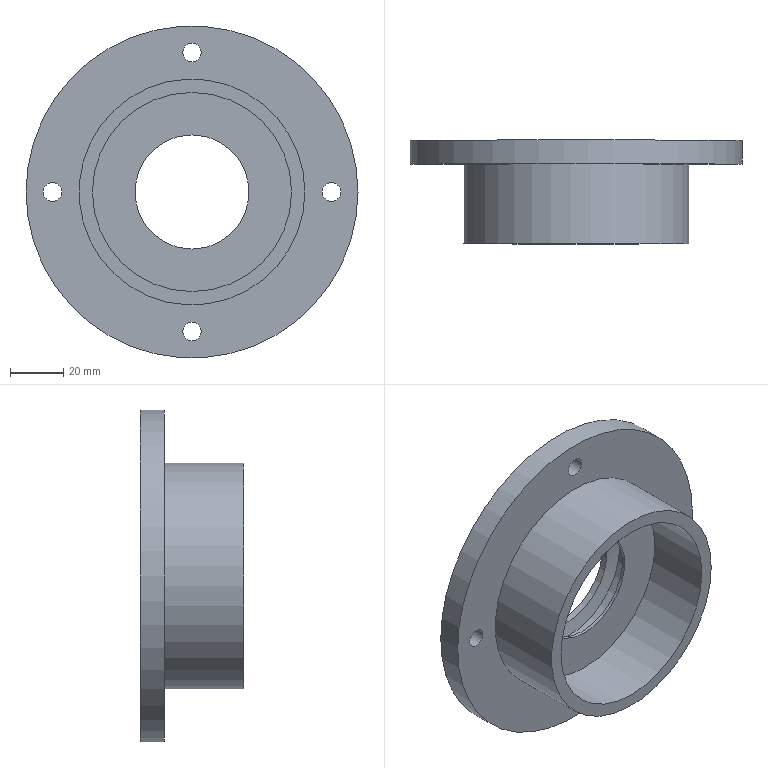Part | NX | features DATUM_CSYS 8, HOLE PACKAGE 7, SIMPLE HOLE 7, SKETCH 7, EXTRACT_DATUM_AXIS 4, Instance Feature 3, EXTRUDE 2, Pattern Feature 1, SWP104 1 | 1 solid | 18 faces | box 125 x 39 x 125 mm | volume 135227 mm3 | cylinder 11 | plane 5 | cone 2 | commonest cylinder face diameters 7 x4 43 x2 54 x1 75 x1 81 x1 85 x1
STEP:
#1=CARTESIAN_POINT('',(0.,-14.,21.5));
#2=VERTEX_POINT('',#1);
#3=CARTESIAN_POINT('',(0.,-14.,0.));
#4=DIRECTION('',(0.,1.,0.));
#5=DIRECTION('',(0.,0.,1.));
#6=AXIS2_PLACEMENT_3D('',#3,#4,#5);
#7=CIRCLE('',#6,21.5);
#8=EDGE_CURVE('',#2,#2,#7,.T.);
#9=ORIENTED_EDGE('',*,*,#8,.F.);
#10=EDGE_LOOP('',(#9));
#11=FACE_BOUND('',#10,.T.);
#12=CARTESIAN_POINT('',(0.,-12.735,21.5));
#13=VERTEX_POINT('',#12);
#14=CARTESIAN_POINT('',(0.,-12.735,0.));
#15=DIRECTION('',(0.,1.,0.));
#16=DIRECTION('',(0.,0.,1.));
#17=AXIS2_PLACEMENT_3D('',#14,#15,#16);
#18=CIRCLE('',#17,21.5);
#19=EDGE_CURVE('',#13,#13,#18,.F.);
#20=ORIENTED_EDGE('',*,*,#19,.F.);
#21=EDGE_LOOP('',(#20));
#22=FACE_BOUND('',#21,.T.);
#23=CARTESIAN_POINT('',(0.,0.,0.));
#24=DIRECTION('',(0.,-1.,0.));
#25=DIRECTION('',(0.,0.,-1.));
#26=AXIS2_PLACEMENT_3D('',#23,#24,#25);
#27=CYLINDRICAL_SURFACE('',#26,21.5);
#28=ADVANCED_FACE('',(#11,#22),#27,.F.);
#29=CARTESIAN_POINT('',(0.,-2.,-21.5));
#30=VERTEX_POINT('',#29);
#31=CARTESIAN_POINT('',(0.,-2.,0.));
#32=DIRECTION('',(0.,-1.,0.));
#33=DIRECTION('',(0.,0.,-1.));
#34=AXIS2_PLACEMENT_3D('',#31,#32,#33);
#35=CIRCLE('',#34,21.5);
#36=EDGE_CURVE('',#30,#30,#35,.T.);
#37=ORIENTED_EDGE('',*,*,#36,.F.);
#38=EDGE_LOOP('',(#37));
#39=FACE_BOUND('',#38,.T.);
#40=CARTESIAN_POINT('',(0.,-4.597,-21.5));
#41=VERTEX_POINT('',#40);
#42=CARTESIAN_POINT('',(0.,-4.597,0.));
#43=DIRECTION('',(0.,-1.,0.));
#44=DIRECTION('',(0.,0.,-1.));
#45=AXIS2_PLACEMENT_3D('',#42,#43,#44);
#46=CIRCLE('',#45,21.5);
#47=EDGE_CURVE('',#41,#41,#46,.F.);
#48=ORIENTED_EDGE('',*,*,#47,.F.);
#49=EDGE_LOOP('',(#48));
#50=FACE_BOUND('',#49,.T.);
#51=CARTESIAN_POINT('',(0.,0.,0.));
#52=DIRECTION('',(0.,-1.,0.));
#53=DIRECTION('',(0.,0.,-1.));
#54=AXIS2_PLACEMENT_3D('',#51,#52,#53);
#55=CYLINDRICAL_SURFACE('',#54,21.5);
#56=ADVANCED_FACE('',(#39,#50),#55,.F.);
#57=CARTESIAN_POINT('',(62.5,-9.,0.));
#58=VERTEX_POINT('',#57);
#59=CARTESIAN_POINT('',(0.,-9.,0.));
#60=DIRECTION('',(0.,-1.,0.));
#61=DIRECTION('',(1.,0.,0.));
#62=AXIS2_PLACEMENT_3D('',#59,#60,#61);
#63=CIRCLE('',#62,62.5);
#64=EDGE_CURVE('',#58,#58,#63,.T.);
#65=ORIENTED_EDGE('',*,*,#64,.F.);
#66=EDGE_LOOP('',(#65));
#67=FACE_BOUND('',#66,.T.);
#68=CARTESIAN_POINT('',(62.5,0.,0.));
#69=VERTEX_POINT('',#68);
#70=CARTESIAN_POINT('',(0.,0.,0.));
#71=DIRECTION('',(0.,-1.,0.));
#72=DIRECTION('',(1.,0.,0.));
#73=AXIS2_PLACEMENT_3D('',#70,#71,#72);
#74=CIRCLE('',#73,62.5);
#75=EDGE_CURVE('',#69,#69,#74,.T.);
#76=ORIENTED_EDGE('',*,*,#75,.T.);
#77=EDGE_LOOP('',(#76));
#78=FACE_BOUND('',#77,.T.);
#79=CARTESIAN_POINT('',(0.,-9.,0.));
#80=DIRECTION('',(0.,1.,0.));
#81=DIRECTION('',(0.,0.,1.));
#82=AXIS2_PLACEMENT_3D('',#79,#80,#81);
#83=CYLINDRICAL_SURFACE('',#82,62.5);
#84=ADVANCED_FACE('',(#67,#78),#83,.T.);
#85=CARTESIAN_POINT('',(0.,-9.,-56.));
#86=VERTEX_POINT('',#85);
#87=CARTESIAN_POINT('',(0.,-9.,-52.5));
#88=DIRECTION('',(0.,-1.,0.));
#89=DIRECTION('',(0.,0.,-1.));
#90=AXIS2_PLACEMENT_3D('',#87,#88,#89);
#91=CIRCLE('',#90,3.5);
#92=EDGE_CURVE('',#86,#86,#91,.T.);
#93=ORIENTED_EDGE('',*,*,#92,.F.);
#94=EDGE_LOOP('',(#93));
#95=FACE_BOUND('',#94,.T.);
#96=CARTESIAN_POINT('',(52.5,-9.,-3.5));
#97=VERTEX_POINT('',#96);
#98=CARTESIAN_POINT('',(52.5,-9.,0.));
#99=DIRECTION('',(0.,-1.,0.));
#100=DIRECTION('',(0.,0.,-1.));
#101=AXIS2_PLACEMENT_3D('',#98,#99,#100);
#102=CIRCLE('',#101,3.5);
#103=EDGE_CURVE('',#97,#97,#102,.T.);
#104=ORIENTED_EDGE('',*,*,#103,.F.);
#105=EDGE_LOOP('',(#104));
#106=FACE_BOUND('',#105,.T.);
#107=CARTESIAN_POINT('',(0.,-9.,49.));
#108=VERTEX_POINT('',#107);
#109=CARTESIAN_POINT('',(0.,-9.,52.5));
#110=DIRECTION('',(0.,-1.,0.));
#111=DIRECTION('',(0.,0.,-1.));
#112=AXIS2_PLACEMENT_3D('',#109,#110,#111);
#113=CIRCLE('',#112,3.5);
#114=EDGE_CURVE('',#108,#108,#113,.T.);
#115=ORIENTED_EDGE('',*,*,#114,.F.);
#116=EDGE_LOOP('',(#115));
#117=FACE_BOUND('',#116,.T.);
#118=CARTESIAN_POINT('',(-52.5,-9.,-3.5));
#119=VERTEX_POINT('',#118);
#120=CARTESIAN_POINT('',(-52.5,-9.,0.));
#121=DIRECTION('',(0.,-1.,0.));
#122=DIRECTION('',(0.,0.,-1.));
#123=AXIS2_PLACEMENT_3D('',#120,#121,#122);
#124=CIRCLE('',#123,3.5);
#125=EDGE_CURVE('',#119,#119,#124,.T.);
#126=ORIENTED_EDGE('',*,*,#125,.F.);
#127=EDGE_LOOP('',(#126));
#128=FACE_BOUND('',#127,.T.);
#129=CARTESIAN_POINT('',(42.5,-9.,0.));
#130=VERTEX_POINT('',#129);
#131=CARTESIAN_POINT('',(0.,-9.,0.));
#132=DIRECTION('',(0.,-1.,0.));
#133=DIRECTION('',(1.,0.,0.));
#134=AXIS2_PLACEMENT_3D('',#131,#132,#133);
#135=CIRCLE('',#134,42.5);
#136=EDGE_CURVE('',#130,#130,#135,.T.);
#137=ORIENTED_EDGE('',*,*,#136,.F.);
#138=EDGE_LOOP('',(#137));
#139=FACE_BOUND('',#138,.T.);
#140=ORIENTED_EDGE('',*,*,#64,.T.);
#141=EDGE_LOOP('',(#140));
#142=FACE_BOUND('',#141,.T.);
#143=CARTESIAN_POINT('',(0.,-9.,0.));
#144=DIRECTION('',(0.,-1.,0.));
#145=DIRECTION('',(0.,0.,-1.));
#146=AXIS2_PLACEMENT_3D('',#143,#144,#145);
#147=PLANE('',#146);
#148=ADVANCED_FACE('',(#95,#106,#117,#128,#139,#142),#147,.T.);
#149=CARTESIAN_POINT('',(0.,0.,-40.5));
#150=VERTEX_POINT('',#149);
#151=CARTESIAN_POINT('',(0.,0.,0.));
#152=DIRECTION('',(0.,-1.,0.));
#153=DIRECTION('',(0.,0.,-1.));
#154=AXIS2_PLACEMENT_3D('',#151,#152,#153);
#155=CIRCLE('',#154,40.5);
#156=EDGE_CURVE('',#150,#150,#155,.T.);
#157=ORIENTED_EDGE('',*,*,#156,.T.);
#158=EDGE_LOOP('',(#157));
#159=FACE_BOUND('',#158,.T.);
#160=CARTESIAN_POINT('',(0.,0.,-56.));
#161=VERTEX_POINT('',#160);
#162=CARTESIAN_POINT('',(0.,0.,-52.5));
#163=DIRECTION('',(0.,-1.,0.));
#164=DIRECTION('',(0.,0.,-1.));
#165=AXIS2_PLACEMENT_3D('',#162,#163,#164);
#166=CIRCLE('',#165,3.5);
#167=EDGE_CURVE('',#161,#161,#166,.T.);
#168=ORIENTED_EDGE('',*,*,#167,.T.);
#169=EDGE_LOOP('',(#168));
#170=FACE_BOUND('',#169,.T.);
#171=CARTESIAN_POINT('',(52.5,0.,-3.5));
#172=VERTEX_POINT('',#171);
#173=CARTESIAN_POINT('',(52.5,0.,0.));
#174=DIRECTION('',(0.,-1.,0.));
#175=DIRECTION('',(0.,0.,-1.));
#176=AXIS2_PLACEMENT_3D('',#173,#174,#175);
#177=CIRCLE('',#176,3.5);
#178=EDGE_CURVE('',#172,#172,#177,.T.);
#179=ORIENTED_EDGE('',*,*,#178,.T.);
#180=EDGE_LOOP('',(#179));
#181=FACE_BOUND('',#180,.T.);
#182=CARTESIAN_POINT('',(0.,0.,49.));
#183=VERTEX_POINT('',#182);
#184=CARTESIAN_POINT('',(0.,0.,52.5));
#185=DIRECTION('',(0.,-1.,0.));
#186=DIRECTION('',(0.,0.,-1.));
#187=AXIS2_PLACEMENT_3D('',#184,#185,#186);
#188=CIRCLE('',#187,3.5);
#189=EDGE_CURVE('',#183,#183,#188,.T.);
#190=ORIENTED_EDGE('',*,*,#189,.T.);
#191=EDGE_LOOP('',(#190));
#192=FACE_BOUND('',#191,.T.);
#193=CARTESIAN_POINT('',(-52.5,0.,-3.5));
#194=VERTEX_POINT('',#193);
#195=CARTESIAN_POINT('',(-52.5,0.,0.));
#196=DIRECTION('',(0.,-1.,0.));
#197=DIRECTION('',(0.,0.,-1.));
#198=AXIS2_PLACEMENT_3D('',#195,#196,#197);
#199=CIRCLE('',#198,3.5);
#200=EDGE_CURVE('',#194,#194,#199,.T.);
#201=ORIENTED_EDGE('',*,*,#200,.T.);
#202=EDGE_LOOP('',(#201));
#203=FACE_BOUND('',#202,.T.);
#204=ORIENTED_EDGE('',*,*,#75,.F.);
#205=EDGE_LOOP('',(#204));
#206=FACE_BOUND('',#205,.T.);
#207=CARTESIAN_POINT('',(0.,0.,0.));
#208=DIRECTION('',(0.,-1.,0.));
#209=DIRECTION('',(0.,0.,-1.));
#210=AXIS2_PLACEMENT_3D('',#207,#208,#209);
#211=PLANE('',#210);
#212=ADVANCED_FACE('',(#159,#170,#181,#192,#203,#206),#211,.F.);
#213=CARTESIAN_POINT('',(42.5,-39.,0.));
#214=VERTEX_POINT('',#213);
#215=CARTESIAN_POINT('',(0.,-39.,0.));
#216=DIRECTION('',(0.,-1.,0.));
#217=DIRECTION('',(1.,0.,0.));
#218=AXIS2_PLACEMENT_3D('',#215,#216,#217);
#219=CIRCLE('',#218,42.5);
#220=EDGE_CURVE('',#214,#214,#219,.T.);
#221=ORIENTED_EDGE('',*,*,#220,.F.);
#222=EDGE_LOOP('',(#221));
#223=FACE_BOUND('',#222,.T.);
#224=ORIENTED_EDGE('',*,*,#136,.T.);
#225=EDGE_LOOP('',(#224));
#226=FACE_BOUND('',#225,.T.);
#227=CARTESIAN_POINT('',(0.,-39.,0.));
#228=DIRECTION('',(0.,1.,0.));
#229=DIRECTION('',(0.,0.,1.));
#230=AXIS2_PLACEMENT_3D('',#227,#228,#229);
#231=CYLINDRICAL_SURFACE('',#230,42.5);
#232=ADVANCED_FACE('',(#223,#226),#231,.T.);
#233=CARTESIAN_POINT('',(0.,-39.,37.5));
#234=VERTEX_POINT('',#233);
#235=CARTESIAN_POINT('',(0.,-39.,0.));
#236=DIRECTION('',(0.,1.,0.));
#237=DIRECTION('',(0.,0.,1.));
#238=AXIS2_PLACEMENT_3D('',#235,#236,#237);
#239=CIRCLE('',#238,37.5);
#240=EDGE_CURVE('',#234,#234,#239,.T.);
#241=ORIENTED_EDGE('',*,*,#240,.T.);
#242=EDGE_LOOP('',(#241));
#243=FACE_BOUND('',#242,.T.);
#244=ORIENTED_EDGE('',*,*,#220,.T.);
#245=EDGE_LOOP('',(#244));
#246=FACE_BOUND('',#245,.T.);
#247=CARTESIAN_POINT('',(0.,-39.,0.));
#248=DIRECTION('',(0.,-1.,0.));
#249=DIRECTION('',(0.,0.,-1.));
#250=AXIS2_PLACEMENT_3D('',#247,#248,#249);
#251=PLANE('',#250);
#252=ADVANCED_FACE('',(#243,#246),#251,.T.);
#253=ORIENTED_EDGE('',*,*,#8,.T.);
#254=EDGE_LOOP('',(#253));
#255=FACE_BOUND('',#254,.T.);
#256=CARTESIAN_POINT('',(0.,-14.,37.5));
#257=VERTEX_POINT('',#256);
#258=CARTESIAN_POINT('',(0.,-14.,0.));
#259=DIRECTION('',(0.,1.,0.));
#260=DIRECTION('',(0.,0.,1.));
#261=AXIS2_PLACEMENT_3D('',#258,#259,#260);
#262=CIRCLE('',#261,37.5);
#263=EDGE_CURVE('',#257,#257,#262,.F.);
#264=ORIENTED_EDGE('',*,*,#263,.T.);
#265=EDGE_LOOP('',(#264));
#266=FACE_BOUND('',#265,.T.);
#267=CARTESIAN_POINT('',(0.,-14.,0.));
#268=DIRECTION('',(0.,1.,0.));
#269=DIRECTION('',(0.,0.,1.));
#270=AXIS2_PLACEMENT_3D('',#267,#268,#269);
#271=PLANE('',#270);
#272=ADVANCED_FACE('',(#255,#266),#271,.F.);
#273=ORIENTED_EDGE('',*,*,#263,.F.);
#274=EDGE_LOOP('',(#273));
#275=FACE_BOUND('',#274,.T.);
#276=ORIENTED_EDGE('',*,*,#240,.F.);
#277=EDGE_LOOP('',(#276));
#278=FACE_BOUND('',#277,.T.);
#279=CARTESIAN_POINT('',(0.,-39.,0.));
#280=DIRECTION('',(0.,1.,0.));
#281=DIRECTION('',(0.,0.,1.));
#282=AXIS2_PLACEMENT_3D('',#279,#280,#281);
#283=CYLINDRICAL_SURFACE('',#282,37.5);
#284=ADVANCED_FACE('',(#275,#278),#283,.F.);
#285=ORIENTED_EDGE('',*,*,#125,.T.);
#286=EDGE_LOOP('',(#285));
#287=FACE_BOUND('',#286,.T.);
#288=ORIENTED_EDGE('',*,*,#200,.F.);
#289=EDGE_LOOP('',(#288));
#290=FACE_BOUND('',#289,.T.);
#291=CARTESIAN_POINT('',(-52.5,0.,0.));
#292=DIRECTION('',(0.,-1.,0.));
#293=DIRECTION('',(0.,0.,-1.));
#294=AXIS2_PLACEMENT_3D('',#291,#292,#293);
#295=CYLINDRICAL_SURFACE('',#294,3.5);
#296=ADVANCED_FACE('',(#287,#290),#295,.F.);
#297=ORIENTED_EDGE('',*,*,#114,.T.);
#298=EDGE_LOOP('',(#297));
#299=FACE_BOUND('',#298,.T.);
#300=ORIENTED_EDGE('',*,*,#189,.F.);
#301=EDGE_LOOP('',(#300));
#302=FACE_BOUND('',#301,.T.);
#303=CARTESIAN_POINT('',(0.,0.,52.5));
#304=DIRECTION('',(0.,-1.,0.));
#305=DIRECTION('',(0.,0.,-1.));
#306=AXIS2_PLACEMENT_3D('',#303,#304,#305);
#307=CYLINDRICAL_SURFACE('',#306,3.5);
#308=ADVANCED_FACE('',(#299,#302),#307,.F.);
#309=ORIENTED_EDGE('',*,*,#103,.T.);
#310=EDGE_LOOP('',(#309));
#311=FACE_BOUND('',#310,.T.);
#312=ORIENTED_EDGE('',*,*,#178,.F.);
#313=EDGE_LOOP('',(#312));
#314=FACE_BOUND('',#313,.T.);
#315=CARTESIAN_POINT('',(52.5,0.,0.));
#316=DIRECTION('',(0.,-1.,0.));
#317=DIRECTION('',(0.,0.,-1.));
#318=AXIS2_PLACEMENT_3D('',#315,#316,#317);
#319=CYLINDRICAL_SURFACE('',#318,3.5);
#320=ADVANCED_FACE('',(#311,#314),#319,.F.);
#321=ORIENTED_EDGE('',*,*,#92,.T.);
#322=EDGE_LOOP('',(#321));
#323=FACE_BOUND('',#322,.T.);
#324=ORIENTED_EDGE('',*,*,#167,.F.);
#325=EDGE_LOOP('',(#324));
#326=FACE_BOUND('',#325,.T.);
#327=CARTESIAN_POINT('',(0.,0.,-52.5));
#328=DIRECTION('',(0.,-1.,0.));
#329=DIRECTION('',(0.,0.,-1.));
#330=AXIS2_PLACEMENT_3D('',#327,#328,#329);
#331=CYLINDRICAL_SURFACE('',#330,3.5);
#332=ADVANCED_FACE('',(#323,#326),#331,.F.);
#333=ORIENTED_EDGE('',*,*,#36,.T.);
#334=EDGE_LOOP('',(#333));
#335=FACE_BOUND('',#334,.T.);
#336=CARTESIAN_POINT('',(0.,-2.,-40.5));
#337=VERTEX_POINT('',#336);
#338=CARTESIAN_POINT('',(0.,-2.,0.));
#339=DIRECTION('',(0.,-1.,0.));
#340=DIRECTION('',(0.,0.,-1.));
#341=AXIS2_PLACEMENT_3D('',#338,#339,#340);
#342=CIRCLE('',#341,40.5);
#343=EDGE_CURVE('',#337,#337,#342,.F.);
#344=ORIENTED_EDGE('',*,*,#343,.T.);
#345=EDGE_LOOP('',(#344));
#346=FACE_BOUND('',#345,.T.);
#347=CARTESIAN_POINT('',(0.,-2.,0.));
#348=DIRECTION('',(0.,-1.,0.));
#349=DIRECTION('',(0.,0.,-1.));
#350=AXIS2_PLACEMENT_3D('',#347,#348,#349);
#351=PLANE('',#350);
#352=ADVANCED_FACE('',(#335,#346),#351,.F.);
#353=ORIENTED_EDGE('',*,*,#343,.F.);
#354=EDGE_LOOP('',(#353));
#355=FACE_BOUND('',#354,.T.);
#356=ORIENTED_EDGE('',*,*,#156,.F.);
#357=EDGE_LOOP('',(#356));
#358=FACE_BOUND('',#357,.T.);
#359=CARTESIAN_POINT('',(0.,0.,0.));
#360=DIRECTION('',(0.,-1.,0.));
#361=DIRECTION('',(0.,0.,-1.));
#362=AXIS2_PLACEMENT_3D('',#359,#360,#361);
#363=CYLINDRICAL_SURFACE('',#362,40.5);
#364=ADVANCED_FACE('',(#355,#358),#363,.F.);
#365=CARTESIAN_POINT('',(0.,-11.666,-27.));
#366=VERTEX_POINT('',#365);
#367=CARTESIAN_POINT('',(0.,-11.666,0.));
#368=DIRECTION('',(0.,-1.,0.));
#369=DIRECTION('',(0.,0.,-1.));
#370=AXIS2_PLACEMENT_3D('',#367,#368,#369);
#371=CIRCLE('',#370,27.);
#372=EDGE_CURVE('',#366,#366,#371,.F.);
#373=ORIENTED_EDGE('',*,*,#372,.T.);
#374=EDGE_LOOP('',(#373));
#375=FACE_BOUND('',#374,.T.);
#376=ORIENTED_EDGE('',*,*,#19,.T.);
#377=EDGE_LOOP('',(#376));
#378=FACE_BOUND('',#377,.T.);
#379=CARTESIAN_POINT('',(0.,-11.666,0.));
#380=DIRECTION('',(0.,1.,0.));
#381=DIRECTION('',(0.,0.,1.));
#382=AXIS2_PLACEMENT_3D('',#379,#380,#381);
#383=CONICAL_SURFACE('',#382,27.,1.379);
#384=ADVANCED_FACE('',(#375,#378),#383,.F.);
#385=CARTESIAN_POINT('',(0.,-5.666,-27.));
#386=VERTEX_POINT('',#385);
#387=CARTESIAN_POINT('',(0.,-5.666,0.));
#388=DIRECTION('',(0.,-1.,0.));
#389=DIRECTION('',(0.,0.,-1.));
#390=AXIS2_PLACEMENT_3D('',#387,#388,#389);
#391=CIRCLE('',#390,27.);
#392=EDGE_CURVE('',#386,#386,#391,.F.);
#393=ORIENTED_EDGE('',*,*,#392,.F.);
#394=EDGE_LOOP('',(#393));
#395=FACE_BOUND('',#394,.T.);
#396=ORIENTED_EDGE('',*,*,#47,.T.);
#397=EDGE_LOOP('',(#396));
#398=FACE_BOUND('',#397,.T.);
#399=CARTESIAN_POINT('',(0.,-4.5,0.));
#400=DIRECTION('',(0.,-1.,0.));
#401=DIRECTION('',(0.,0.,-1.));
#402=AXIS2_PLACEMENT_3D('',#399,#400,#401);
#403=CONICAL_SURFACE('',#402,21.,1.379);
#404=ADVANCED_FACE('',(#395,#398),#403,.F.);
#405=ORIENTED_EDGE('',*,*,#372,.F.);
#406=EDGE_LOOP('',(#405));
#407=FACE_BOUND('',#406,.T.);
#408=ORIENTED_EDGE('',*,*,#392,.T.);
#409=EDGE_LOOP('',(#408));
#410=FACE_BOUND('',#409,.T.);
#411=CARTESIAN_POINT('',(0.,-2.,0.));
#412=DIRECTION('',(0.,-1.,0.));
#413=DIRECTION('',(0.,0.,-1.));
#414=AXIS2_PLACEMENT_3D('',#411,#412,#413);
#415=CYLINDRICAL_SURFACE('',#414,27.);
#416=ADVANCED_FACE('',(#407,#410),#415,.F.);
#417=CLOSED_SHELL('',(#28,#56,#84,#148,#212,#232,#252,#272,#284,#296,#308,#320,#332,#352,#364,#384,#404,#416));
#418=MANIFOLD_SOLID_BREP('',#417);
#419=(LENGTH_UNIT()NAMED_UNIT(*)SI_UNIT(.MILLI.,.METRE.));
#420=UNCERTAINTY_MEASURE_WITH_UNIT(LENGTH_MEASURE(0.00001),#419,'','');
#421=(NAMED_UNIT(*)PLANE_ANGLE_UNIT()SI_UNIT($,.RADIAN.));
#422=(NAMED_UNIT(*)SI_UNIT($,.STERADIAN.)SOLID_ANGLE_UNIT());
#423=(GEOMETRIC_REPRESENTATION_CONTEXT(3)GLOBAL_UNCERTAINTY_ASSIGNED_CONTEXT((#420))GLOBAL_UNIT_ASSIGNED_CONTEXT((#419,#421,#422))REPRESENTATION_CONTEXT('',''));
#424=ADVANCED_BREP_SHAPE_REPRESENTATION('',(#418),#423);